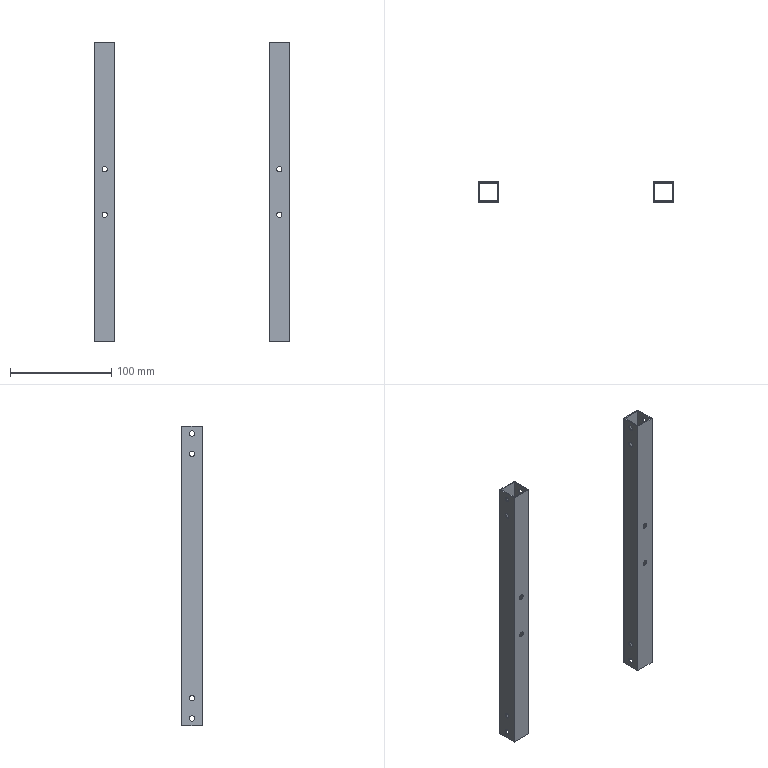Part | SolidWorks | features BaseBody 2 | 2 solids | 68 faces | box 193 x 20 x 296 mm | volume 44469 mm3 | cylinder 48 | plane 20 | commonest cylinder face diameters 5.3 x32 5.2 x16